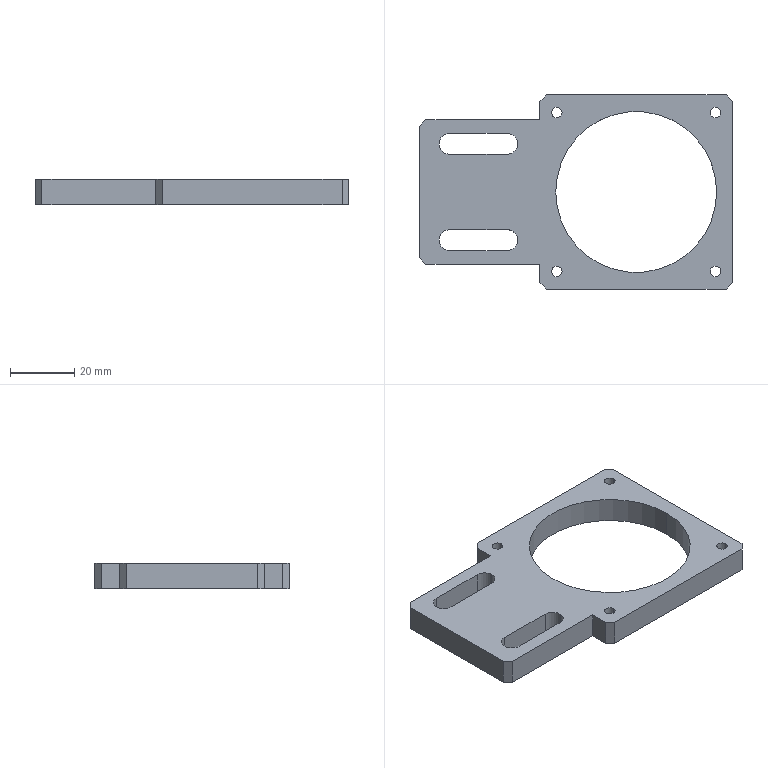Part | 1 solid | 44 faces | box 97.5 x 60.5 x 8 mm | volume 23818 mm3 | cylinder 20 | plane 20 | cone 4 | commonest cylinder face diameters 3.3 x12 6.5 x6 50.1 x2
STEP:
#1=CARTESIAN_POINT('',(-18.153,-15.,0.));
#2=VERTEX_POINT('',#1);
#3=CARTESIAN_POINT('',(-21.403,-18.25,0.));
#4=VERTEX_POINT('',#3);
#5=CARTESIAN_POINT('',(-21.403,-15.,0.));
#6=DIRECTION('',(0.,0.,-1.));
#7=DIRECTION('',(-1.,0.,0.));
#8=AXIS2_PLACEMENT_3D('',#5,#6,#7);
#9=CIRCLE('',#8,3.25);
#10=EDGE_CURVE('',#2,#4,#9,.T.);
#11=ORIENTED_EDGE('',*,*,#10,.F.);
#12=CARTESIAN_POINT('',(-18.153,-15.,-8.));
#13=VERTEX_POINT('',#12);
#14=CARTESIAN_POINT('',(-18.153,-15.,0.));
#15=DIRECTION('',(0.,0.,-1.));
#16=VECTOR('',#15,1000.);
#17=LINE('',#14,#16);
#18=EDGE_CURVE('',#2,#13,#17,.T.);
#19=ORIENTED_EDGE('',*,*,#18,.T.);
#20=CARTESIAN_POINT('',(-21.403,-18.25,-8.));
#21=VERTEX_POINT('',#20);
#22=CARTESIAN_POINT('',(-21.403,-15.,-8.));
#23=DIRECTION('',(0.,0.,-1.));
#24=DIRECTION('',(-1.,0.,0.));
#25=AXIS2_PLACEMENT_3D('',#22,#23,#24);
#26=CIRCLE('',#25,3.25);
#27=EDGE_CURVE('',#13,#21,#26,.T.);
#28=ORIENTED_EDGE('',*,*,#27,.T.);
#29=CARTESIAN_POINT('',(-21.403,-18.25,0.));
#30=DIRECTION('',(0.,0.,-1.));
#31=VECTOR('',#30,1000.);
#32=LINE('',#29,#31);
#33=EDGE_CURVE('',#4,#21,#32,.T.);
#34=ORIENTED_EDGE('',*,*,#33,.F.);
#35=EDGE_LOOP('',(#11,#19,#28,#34));
#36=FACE_BOUND('',#35,.T.);
#37=CARTESIAN_POINT('',(-21.403,-15.,0.));
#38=DIRECTION('',(0.,0.,-1.));
#39=DIRECTION('',(-1.,0.,0.));
#40=AXIS2_PLACEMENT_3D('',#37,#38,#39);
#41=CYLINDRICAL_SURFACE('',#40,3.25);
#42=ADVANCED_FACE('',(#36),#41,.F.);
#43=CARTESIAN_POINT('',(-18.153,15.,0.));
#44=VERTEX_POINT('',#43);
#45=CARTESIAN_POINT('',(-21.403,11.75,0.));
#46=VERTEX_POINT('',#45);
#47=CARTESIAN_POINT('',(-21.403,15.,0.));
#48=DIRECTION('',(0.,0.,-1.));
#49=DIRECTION('',(1.,0.,0.));
#50=AXIS2_PLACEMENT_3D('',#47,#48,#49);
#51=CIRCLE('',#50,3.25);
#52=EDGE_CURVE('',#44,#46,#51,.T.);
#53=ORIENTED_EDGE('',*,*,#52,.F.);
#54=CARTESIAN_POINT('',(-18.153,15.,-8.));
#55=VERTEX_POINT('',#54);
#56=CARTESIAN_POINT('',(-18.153,15.,0.));
#57=DIRECTION('',(0.,0.,-1.));
#58=VECTOR('',#57,1000.);
#59=LINE('',#56,#58);
#60=EDGE_CURVE('',#44,#55,#59,.T.);
#61=ORIENTED_EDGE('',*,*,#60,.T.);
#62=CARTESIAN_POINT('',(-21.403,11.75,-8.));
#63=VERTEX_POINT('',#62);
#64=CARTESIAN_POINT('',(-21.403,15.,-8.));
#65=DIRECTION('',(0.,0.,-1.));
#66=DIRECTION('',(1.,0.,0.));
#67=AXIS2_PLACEMENT_3D('',#64,#65,#66);
#68=CIRCLE('',#67,3.25);
#69=EDGE_CURVE('',#55,#63,#68,.T.);
#70=ORIENTED_EDGE('',*,*,#69,.T.);
#71=CARTESIAN_POINT('',(-21.403,11.75,0.));
#72=DIRECTION('',(0.,0.,-1.));
#73=VECTOR('',#72,1000.);
#74=LINE('',#71,#73);
#75=EDGE_CURVE('',#46,#63,#74,.T.);
#76=ORIENTED_EDGE('',*,*,#75,.F.);
#77=EDGE_LOOP('',(#53,#61,#70,#76));
#78=FACE_BOUND('',#77,.T.);
#79=CARTESIAN_POINT('',(-21.403,15.,0.));
#80=DIRECTION('',(0.,0.,-1.));
#81=DIRECTION('',(-1.,0.,0.));
#82=AXIS2_PLACEMENT_3D('',#79,#80,#81);
#83=CYLINDRICAL_SURFACE('',#82,3.25);
#84=ADVANCED_FACE('',(#78),#83,.F.);
#85=CARTESIAN_POINT('',(38.65,-21.65,-5.5));
#86=VERTEX_POINT('',#85);
#87=CARTESIAN_POINT('',(38.65,-18.35,-5.5));
#88=VERTEX_POINT('',#87);
#89=CARTESIAN_POINT('',(38.65,-20.,-5.5));
#90=DIRECTION('',(1.,0.,0.));
#91=DIRECTION('',(0.,1.,0.));
#92=AXIS2_PLACEMENT_3D('',#89,#90,#91);
#93=CIRCLE('',#92,1.65);
#94=EDGE_CURVE('',#86,#88,#93,.T.);
#95=ORIENTED_EDGE('',*,*,#94,.F.);
#96=CARTESIAN_POINT('',(48.75,-21.65,-5.5));
#97=VERTEX_POINT('',#96);
#98=CARTESIAN_POINT('',(48.75,-21.65,-5.5));
#99=DIRECTION('',(1.,0.,0.));
#100=VECTOR('',#99,1000.);
#101=LINE('',#98,#100);
#102=EDGE_CURVE('',#97,#86,#101,.F.);
#103=ORIENTED_EDGE('',*,*,#102,.F.);
#104=CARTESIAN_POINT('',(48.75,-18.35,-5.5));
#105=VERTEX_POINT('',#104);
#106=CARTESIAN_POINT('',(48.75,-20.,-5.5));
#107=DIRECTION('',(1.,0.,0.));
#108=DIRECTION('',(0.,1.,0.));
#109=AXIS2_PLACEMENT_3D('',#106,#107,#108);
#110=CIRCLE('',#109,1.65);
#111=EDGE_CURVE('',#97,#105,#110,.T.);
#112=ORIENTED_EDGE('',*,*,#111,.T.);
#113=CARTESIAN_POINT('',(48.75,-18.35,-5.5));
#114=DIRECTION('',(1.,0.,0.));
#115=VECTOR('',#114,1000.);
#116=LINE('',#113,#115);
#117=EDGE_CURVE('',#105,#88,#116,.F.);
#118=ORIENTED_EDGE('',*,*,#117,.T.);
#119=EDGE_LOOP('',(#95,#103,#112,#118));
#120=FACE_BOUND('',#119,.T.);
#121=CARTESIAN_POINT('',(48.75,-20.,-5.5));
#122=DIRECTION('',(1.,0.,0.));
#123=DIRECTION('',(0.,-1.,0.));
#124=AXIS2_PLACEMENT_3D('',#121,#122,#123);
#125=CYLINDRICAL_SURFACE('',#124,1.65);
#126=ADVANCED_FACE('',(#120),#125,.F.);
#127=CARTESIAN_POINT('',(37.659,-20.,-5.5));
#128=VERTEX_POINT('',#127);
#129=CARTESIAN_POINT('',(38.65,-18.35,-5.5));
#130=DIRECTION('',(0.515,0.8572,0.));
#131=VECTOR('',#130,1000.);
#132=LINE('',#129,#131);
#133=EDGE_CURVE('',#88,#128,#132,.F.);
#134=ORIENTED_EDGE('',*,*,#133,.T.);
#135=CARTESIAN_POINT('',(38.65,-21.65,-5.5));
#136=DIRECTION('',(0.515,-0.8572,0.));
#137=VECTOR('',#136,1000.);
#138=LINE('',#135,#137);
#139=EDGE_CURVE('',#86,#128,#138,.F.);
#140=ORIENTED_EDGE('',*,*,#139,.F.);
#141=ORIENTED_EDGE('',*,*,#94,.T.);
#142=EDGE_LOOP('',(#134,#140,#141));
#143=FACE_BOUND('',#142,.T.);
#144=CARTESIAN_POINT('',(38.65,-20.,-5.5));
#145=DIRECTION('',(1.,0.,0.));
#146=DIRECTION('',(0.,-1.,0.));
#147=AXIS2_PLACEMENT_3D('',#144,#145,#146);
#148=CONICAL_SURFACE('',#147,1.65,1.03);
#149=ADVANCED_FACE('',(#143),#148,.F.);
#150=CARTESIAN_POINT('',(38.65,18.35,-5.5));
#151=VERTEX_POINT('',#150);
#152=CARTESIAN_POINT('',(38.65,21.65,-5.5));
#153=VERTEX_POINT('',#152);
#154=CARTESIAN_POINT('',(38.65,20.,-5.5));
#155=DIRECTION('',(1.,0.,0.));
#156=DIRECTION('',(0.,1.,0.));
#157=AXIS2_PLACEMENT_3D('',#154,#155,#156);
#158=CIRCLE('',#157,1.65);
#159=EDGE_CURVE('',#151,#153,#158,.T.);
#160=ORIENTED_EDGE('',*,*,#159,.F.);
#161=CARTESIAN_POINT('',(48.75,18.35,-5.5));
#162=VERTEX_POINT('',#161);
#163=CARTESIAN_POINT('',(48.75,18.35,-5.5));
#164=DIRECTION('',(1.,0.,0.));
#165=VECTOR('',#164,1000.);
#166=LINE('',#163,#165);
#167=EDGE_CURVE('',#162,#151,#166,.F.);
#168=ORIENTED_EDGE('',*,*,#167,.F.);
#169=CARTESIAN_POINT('',(48.75,21.65,-5.5));
#170=VERTEX_POINT('',#169);
#171=CARTESIAN_POINT('',(48.75,20.,-5.5));
#172=DIRECTION('',(1.,0.,0.));
#173=DIRECTION('',(0.,1.,0.));
#174=AXIS2_PLACEMENT_3D('',#171,#172,#173);
#175=CIRCLE('',#174,1.65);
#176=EDGE_CURVE('',#162,#170,#175,.T.);
#177=ORIENTED_EDGE('',*,*,#176,.T.);
#178=CARTESIAN_POINT('',(48.75,21.65,-5.5));
#179=DIRECTION('',(1.,0.,0.));
#180=VECTOR('',#179,1000.);
#181=LINE('',#178,#180);
#182=EDGE_CURVE('',#170,#153,#181,.F.);
#183=ORIENTED_EDGE('',*,*,#182,.T.);
#184=EDGE_LOOP('',(#160,#168,#177,#183));
#185=FACE_BOUND('',#184,.T.);
#186=CARTESIAN_POINT('',(48.75,20.,-5.5));
#187=DIRECTION('',(1.,0.,0.));
#188=DIRECTION('',(0.,-1.,0.));
#189=AXIS2_PLACEMENT_3D('',#186,#187,#188);
#190=CYLINDRICAL_SURFACE('',#189,1.65);
#191=ADVANCED_FACE('',(#185),#190,.F.);
#192=CARTESIAN_POINT('',(37.659,20.,-5.5));
#193=VERTEX_POINT('',#192);
#194=CARTESIAN_POINT('',(38.65,21.65,-5.5));
#195=DIRECTION('',(0.515,0.8572,0.));
#196=VECTOR('',#195,1000.);
#197=LINE('',#194,#196);
#198=EDGE_CURVE('',#153,#193,#197,.F.);
#199=ORIENTED_EDGE('',*,*,#198,.T.);
#200=CARTESIAN_POINT('',(38.65,18.35,-5.5));
#201=DIRECTION('',(0.515,-0.8572,0.));
#202=VECTOR('',#201,1000.);
#203=LINE('',#200,#202);
#204=EDGE_CURVE('',#151,#193,#203,.F.);
#205=ORIENTED_EDGE('',*,*,#204,.F.);
#206=ORIENTED_EDGE('',*,*,#159,.T.);
#207=EDGE_LOOP('',(#199,#205,#206));
#208=FACE_BOUND('',#207,.T.);
#209=CARTESIAN_POINT('',(38.65,20.,-5.5));
#210=DIRECTION('',(1.,0.,0.));
#211=DIRECTION('',(0.,-1.,0.));
#212=AXIS2_PLACEMENT_3D('',#209,#210,#211);
#213=CONICAL_SURFACE('',#212,1.65,1.03);
#214=ADVANCED_FACE('',(#208),#213,.F.);
#215=CARTESIAN_POINT('',(-6.3,0.,0.));
#216=VERTEX_POINT('',#215);
#217=CARTESIAN_POINT('',(43.8,0.,0.));
#218=VERTEX_POINT('',#217);
#219=CARTESIAN_POINT('',(18.75,0.,0.));
#220=DIRECTION('',(0.,0.,-1.));
#221=DIRECTION('',(1.,0.,0.));
#222=AXIS2_PLACEMENT_3D('',#219,#220,#221);
#223=CIRCLE('',#222,25.05);
#224=EDGE_CURVE('',#216,#218,#223,.T.);
#225=ORIENTED_EDGE('',*,*,#224,.F.);
#226=CARTESIAN_POINT('',(-6.3,0.,-8.));
#227=VERTEX_POINT('',#226);
#228=CARTESIAN_POINT('',(-6.3,0.,0.));
#229=DIRECTION('',(0.,0.,-1.));
#230=VECTOR('',#229,1000.);
#231=LINE('',#228,#230);
#232=EDGE_CURVE('',#227,#216,#231,.F.);
#233=ORIENTED_EDGE('',*,*,#232,.F.);
#234=CARTESIAN_POINT('',(43.8,0.,-8.));
#235=VERTEX_POINT('',#234);
#236=CARTESIAN_POINT('',(18.75,0.,-8.));
#237=DIRECTION('',(0.,0.,-1.));
#238=DIRECTION('',(1.,0.,0.));
#239=AXIS2_PLACEMENT_3D('',#236,#237,#238);
#240=CIRCLE('',#239,25.05);
#241=EDGE_CURVE('',#227,#235,#240,.T.);
#242=ORIENTED_EDGE('',*,*,#241,.T.);
#243=CARTESIAN_POINT('',(43.8,0.,0.));
#244=DIRECTION('',(0.,0.,-1.));
#245=VECTOR('',#244,1000.);
#246=LINE('',#243,#245);
#247=EDGE_CURVE('',#235,#218,#246,.F.);
#248=ORIENTED_EDGE('',*,*,#247,.T.);
#249=EDGE_LOOP('',(#225,#233,#242,#248));
#250=FACE_BOUND('',#249,.T.);
#251=CARTESIAN_POINT('',(18.75,0.,0.));
#252=DIRECTION('',(0.,0.,-1.));
#253=DIRECTION('',(-1.,0.,0.));
#254=AXIS2_PLACEMENT_3D('',#251,#252,#253);
#255=CYLINDRICAL_SURFACE('',#254,25.05);
#256=ADVANCED_FACE('',(#250),#255,.F.);
#257=CARTESIAN_POINT('',(45.149,24.749,0.));
#258=VERTEX_POINT('',#257);
#259=CARTESIAN_POINT('',(41.849,24.749,0.));
#260=VERTEX_POINT('',#259);
#261=CARTESIAN_POINT('',(43.499,24.749,0.));
#262=DIRECTION('',(0.,0.,1.));
#263=DIRECTION('',(-1.,0.,0.));
#264=AXIS2_PLACEMENT_3D('',#261,#262,#263);
#265=CIRCLE('',#264,1.65);
#266=EDGE_CURVE('',#258,#260,#265,.T.);
#267=ORIENTED_EDGE('',*,*,#266,.T.);
#268=CARTESIAN_POINT('',(41.849,24.749,-8.));
#269=VERTEX_POINT('',#268);
#270=CARTESIAN_POINT('',(41.849,24.749,-8.));
#271=DIRECTION('',(0.,0.,-1.));
#272=VECTOR('',#271,1000.);
#273=LINE('',#270,#272);
#274=EDGE_CURVE('',#269,#260,#273,.F.);
#275=ORIENTED_EDGE('',*,*,#274,.F.);
#276=CARTESIAN_POINT('',(45.149,24.749,-8.));
#277=VERTEX_POINT('',#276);
#278=CARTESIAN_POINT('',(43.499,24.749,-8.));
#279=DIRECTION('',(0.,0.,-1.));
#280=DIRECTION('',(1.,0.,0.));
#281=AXIS2_PLACEMENT_3D('',#278,#279,#280);
#282=CIRCLE('',#281,1.65);
#283=EDGE_CURVE('',#269,#277,#282,.T.);
#284=ORIENTED_EDGE('',*,*,#283,.T.);
#285=CARTESIAN_POINT('',(45.149,24.749,-8.));
#286=DIRECTION('',(0.,0.,-1.));
#287=VECTOR('',#286,1000.);
#288=LINE('',#285,#287);
#289=EDGE_CURVE('',#277,#258,#288,.F.);
#290=ORIENTED_EDGE('',*,*,#289,.T.);
#291=EDGE_LOOP('',(#267,#275,#284,#290));
#292=FACE_BOUND('',#291,.T.);
#293=CARTESIAN_POINT('',(43.499,24.749,-8.));
#294=DIRECTION('',(0.,0.,-1.));
#295=DIRECTION('',(-1.,0.,0.));
#296=AXIS2_PLACEMENT_3D('',#293,#294,#295);
#297=CYLINDRICAL_SURFACE('',#296,1.65);
#298=ADVANCED_FACE('',(#292),#297,.F.);
#299=CARTESIAN_POINT('',(45.149,-24.749,0.));
#300=VERTEX_POINT('',#299);
#301=CARTESIAN_POINT('',(41.849,-24.749,0.));
#302=VERTEX_POINT('',#301);
#303=CARTESIAN_POINT('',(43.499,-24.749,0.));
#304=DIRECTION('',(0.,0.,1.));
#305=DIRECTION('',(-1.,0.,0.));
#306=AXIS2_PLACEMENT_3D('',#303,#304,#305);
#307=CIRCLE('',#306,1.65);
#308=EDGE_CURVE('',#300,#302,#307,.T.);
#309=ORIENTED_EDGE('',*,*,#308,.T.);
#310=CARTESIAN_POINT('',(41.849,-24.749,-8.));
#311=VERTEX_POINT('',#310);
#312=CARTESIAN_POINT('',(41.849,-24.749,-8.));
#313=DIRECTION('',(0.,0.,-1.));
#314=VECTOR('',#313,1000.);
#315=LINE('',#312,#314);
#316=EDGE_CURVE('',#311,#302,#315,.F.);
#317=ORIENTED_EDGE('',*,*,#316,.F.);
#318=CARTESIAN_POINT('',(45.149,-24.749,-8.));
#319=VERTEX_POINT('',#318);
#320=CARTESIAN_POINT('',(43.499,-24.749,-8.));
#321=DIRECTION('',(0.,0.,-1.));
#322=DIRECTION('',(1.,0.,0.));
#323=AXIS2_PLACEMENT_3D('',#320,#321,#322);
#324=CIRCLE('',#323,1.65);
#325=EDGE_CURVE('',#311,#319,#324,.T.);
#326=ORIENTED_EDGE('',*,*,#325,.T.);
#327=CARTESIAN_POINT('',(45.149,-24.749,-8.));
#328=DIRECTION('',(0.,0.,-1.));
#329=VECTOR('',#328,1000.);
#330=LINE('',#327,#329);
#331=EDGE_CURVE('',#319,#300,#330,.F.);
#332=ORIENTED_EDGE('',*,*,#331,.T.);
#333=EDGE_LOOP('',(#309,#317,#326,#332));
#334=FACE_BOUND('',#333,.T.);
#335=CARTESIAN_POINT('',(43.499,-24.749,-8.));
#336=DIRECTION('',(0.,0.,-1.));
#337=DIRECTION('',(-1.,0.,0.));
#338=AXIS2_PLACEMENT_3D('',#335,#336,#337);
#339=CYLINDRICAL_SURFACE('',#338,1.65);
#340=ADVANCED_FACE('',(#334),#339,.F.);
#341=CARTESIAN_POINT('',(-4.349,-24.749,0.));
#342=VERTEX_POINT('',#341);
#343=CARTESIAN_POINT('',(-7.649,-24.749,0.));
#344=VERTEX_POINT('',#343);
#345=CARTESIAN_POINT('',(-5.999,-24.749,0.));
#346=DIRECTION('',(0.,0.,1.));
#347=DIRECTION('',(-1.,0.,0.));
#348=AXIS2_PLACEMENT_3D('',#345,#346,#347);
#349=CIRCLE('',#348,1.65);
#350=EDGE_CURVE('',#342,#344,#349,.T.);
#351=ORIENTED_EDGE('',*,*,#350,.T.);
#352=CARTESIAN_POINT('',(-7.649,-24.749,-8.));
#353=VERTEX_POINT('',#352);
#354=CARTESIAN_POINT('',(-7.649,-24.749,-8.));
#355=DIRECTION('',(0.,0.,-1.));
#356=VECTOR('',#355,1000.);
#357=LINE('',#354,#356);
#358=EDGE_CURVE('',#353,#344,#357,.F.);
#359=ORIENTED_EDGE('',*,*,#358,.F.);
#360=CARTESIAN_POINT('',(-4.349,-24.749,-8.));
#361=VERTEX_POINT('',#360);
#362=CARTESIAN_POINT('',(-5.999,-24.749,-8.));
#363=DIRECTION('',(0.,0.,-1.));
#364=DIRECTION('',(1.,0.,0.));
#365=AXIS2_PLACEMENT_3D('',#362,#363,#364);
#366=CIRCLE('',#365,1.65);
#367=EDGE_CURVE('',#353,#361,#366,.T.);
#368=ORIENTED_EDGE('',*,*,#367,.T.);
#369=CARTESIAN_POINT('',(-4.349,-24.749,-8.));
#370=DIRECTION('',(0.,0.,-1.));
#371=VECTOR('',#370,1000.);
#372=LINE('',#369,#371);
#373=EDGE_CURVE('',#361,#342,#372,.F.);
#374=ORIENTED_EDGE('',*,*,#373,.T.);
#375=EDGE_LOOP('',(#351,#359,#368,#374));
#376=FACE_BOUND('',#375,.T.);
#377=CARTESIAN_POINT('',(-5.999,-24.749,-8.));
#378=DIRECTION('',(0.,0.,-1.));
#379=DIRECTION('',(-1.,0.,0.));
#380=AXIS2_PLACEMENT_3D('',#377,#378,#379);
#381=CYLINDRICAL_SURFACE('',#380,1.65);
#382=ADVANCED_FACE('',(#376),#381,.F.);
#383=CARTESIAN_POINT('',(-4.349,24.749,0.));
#384=VERTEX_POINT('',#383);
#385=CARTESIAN_POINT('',(-7.649,24.749,0.));
#386=VERTEX_POINT('',#385);
#387=CARTESIAN_POINT('',(-5.999,24.749,0.));
#388=DIRECTION('',(0.,0.,1.));
#389=DIRECTION('',(-1.,0.,0.));
#390=AXIS2_PLACEMENT_3D('',#387,#388,#389);
#391=CIRCLE('',#390,1.65);
#392=EDGE_CURVE('',#384,#386,#391,.T.);
#393=ORIENTED_EDGE('',*,*,#392,.T.);
#394=CARTESIAN_POINT('',(-7.649,24.749,-8.));
#395=VERTEX_POINT('',#394);
#396=CARTESIAN_POINT('',(-7.649,24.749,-8.));
#397=DIRECTION('',(0.,0.,-1.));
#398=VECTOR('',#397,1000.);
#399=LINE('',#396,#398);
#400=EDGE_CURVE('',#395,#386,#399,.F.);
#401=ORIENTED_EDGE('',*,*,#400,.F.);
#402=CARTESIAN_POINT('',(-4.349,24.749,-8.));
#403=VERTEX_POINT('',#402);
#404=CARTESIAN_POINT('',(-5.999,24.749,-8.));
#405=DIRECTION('',(0.,0.,-1.));
#406=DIRECTION('',(1.,0.,0.));
#407=AXIS2_PLACEMENT_3D('',#404,#405,#406);
#408=CIRCLE('',#407,1.65);
#409=EDGE_CURVE('',#395,#403,#408,.T.);
#410=ORIENTED_EDGE('',*,*,#409,.T.);
#411=CARTESIAN_POINT('',(-4.349,24.749,-8.));
#412=DIRECTION('',(0.,0.,-1.));
#413=VECTOR('',#412,1000.);
#414=LINE('',#411,#413);
#415=EDGE_CURVE('',#403,#384,#414,.F.);
#416=ORIENTED_EDGE('',*,*,#415,.T.);
#417=EDGE_LOOP('',(#393,#401,#410,#416));
#418=FACE_BOUND('',#417,.T.);
#419=CARTESIAN_POINT('',(-5.999,24.749,-8.));
#420=DIRECTION('',(0.,0.,-1.));
#421=DIRECTION('',(-1.,0.,0.));
#422=AXIS2_PLACEMENT_3D('',#419,#420,#421);
#423=CYLINDRICAL_SURFACE('',#422,1.65);
#424=ADVANCED_FACE('',(#418),#423,.F.);
#425=CARTESIAN_POINT('',(-39.403,-11.75,-8.));
#426=VERTEX_POINT('',#425);
#427=CARTESIAN_POINT('',(-21.403,-11.75,-8.));
#428=VERTEX_POINT('',#427);
#429=CARTESIAN_POINT('',(-39.403,-11.75,-8.));
#430=DIRECTION('',(1.,0.,0.));
#431=VECTOR('',#430,1000.);
#432=LINE('',#429,#431);
#433=EDGE_CURVE('',#426,#428,#432,.T.);
#434=ORIENTED_EDGE('',*,*,#433,.F.);
#435=CARTESIAN_POINT('',(-39.403,-18.25,-8.));
#436=VERTEX_POINT('',#435);
#437=CARTESIAN_POINT('',(-39.403,-15.,-8.));
#438=DIRECTION('',(0.,0.,-1.));
#439=DIRECTION('',(-1.,0.,0.));
#440=AXIS2_PLACEMENT_3D('',#437,#438,#439);
#441=CIRCLE('',#440,3.25);
#442=EDGE_CURVE('',#436,#426,#441,.T.);
#443=ORIENTED_EDGE('',*,*,#442,.F.);
#444=CARTESIAN_POINT('',(-39.403,-18.25,-8.));
#445=DIRECTION('',(-1.,0.,0.));
#446=VECTOR('',#445,1000.);
#447=LINE('',#444,#446);
#448=EDGE_CURVE('',#21,#436,#447,.T.);
#449=ORIENTED_EDGE('',*,*,#448,.F.);
#450=ORIENTED_EDGE('',*,*,#27,.F.);
#451=CARTESIAN_POINT('',(-21.403,-15.,-8.));
#452=DIRECTION('',(0.,0.,-1.));
#453=DIRECTION('',(-1.,0.,0.));
#454=AXIS2_PLACEMENT_3D('',#451,#452,#453);
#455=CIRCLE('',#454,3.25);
#456=EDGE_CURVE('',#428,#13,#455,.T.);
#457=ORIENTED_EDGE('',*,*,#456,.F.);
#458=EDGE_LOOP('',(#434,#443,#449,#450,#457));
#459=FACE_BOUND('',#458,.T.);
#460=CARTESIAN_POINT('',(-39.403,18.25,-8.));
#461=VERTEX_POINT('',#460);
#462=CARTESIAN_POINT('',(-21.403,18.25,-8.));
#463=VERTEX_POINT('',#462);
#464=CARTESIAN_POINT('',(-39.403,18.25,-8.));
#465=DIRECTION('',(1.,0.,0.));
#466=VECTOR('',#465,1000.);
#467=LINE('',#464,#466);
#468=EDGE_CURVE('',#461,#463,#467,.T.);
#469=ORIENTED_EDGE('',*,*,#468,.F.);
#470=CARTESIAN_POINT('',(-39.403,11.75,-8.));
#471=VERTEX_POINT('',#470);
#472=CARTESIAN_POINT('',(-39.403,15.,-8.));
#473=DIRECTION('',(0.,0.,-1.));
#474=DIRECTION('',(1.,0.,0.));
#475=AXIS2_PLACEMENT_3D('',#472,#473,#474);
#476=CIRCLE('',#475,3.25);
#477=EDGE_CURVE('',#471,#461,#476,.T.);
#478=ORIENTED_EDGE('',*,*,#477,.F.);
#479=CARTESIAN_POINT('',(-39.403,11.75,-8.));
#480=DIRECTION('',(-1.,0.,0.));
#481=VECTOR('',#480,1000.);
#482=LINE('',#479,#481);
#483=EDGE_CURVE('',#63,#471,#482,.T.);
#484=ORIENTED_EDGE('',*,*,#483,.F.);
#485=ORIENTED_EDGE('',*,*,#69,.F.);
#486=CARTESIAN_POINT('',(-21.403,15.,-8.));
#487=DIRECTION('',(0.,0.,-1.));
#488=DIRECTION('',(1.,0.,0.));
#489=AXIS2_PLACEMENT_3D('',#486,#487,#488);
#490=CIRCLE('',#489,3.25);
#491=EDGE_CURVE('',#463,#55,#490,.T.);
#492=ORIENTED_EDGE('',*,*,#491,.F.);
#493=EDGE_LOOP('',(#469,#478,#484,#485,#492));
#494=FACE_BOUND('',#493,.T.);
#495=CARTESIAN_POINT('',(18.75,0.,-8.));
#496=DIRECTION('',(0.,0.,-1.));
#497=DIRECTION('',(1.,0.,0.));
#498=AXIS2_PLACEMENT_3D('',#495,#496,#497);
#499=CIRCLE('',#498,25.05);
#500=EDGE_CURVE('',#235,#227,#499,.T.);
#501=ORIENTED_EDGE('',*,*,#500,.F.);
#502=ORIENTED_EDGE('',*,*,#241,.F.);
#503=EDGE_LOOP('',(#501,#502));
#504=FACE_BOUND('',#503,.T.);
#505=CARTESIAN_POINT('',(43.499,24.749,-8.));
#506=DIRECTION('',(0.,0.,-1.));
#507=DIRECTION('',(1.,0.,0.));
#508=AXIS2_PLACEMENT_3D('',#505,#506,#507);
#509=CIRCLE('',#508,1.65);
#510=EDGE_CURVE('',#277,#269,#509,.T.);
#511=ORIENTED_EDGE('',*,*,#510,.F.);
#512=ORIENTED_EDGE('',*,*,#283,.F.);
#513=EDGE_LOOP('',(#511,#512));
#514=FACE_BOUND('',#513,.T.);
#515=CARTESIAN_POINT('',(43.499,-24.749,-8.));
#516=DIRECTION('',(0.,0.,-1.));
#517=DIRECTION('',(1.,0.,0.));
#518=AXIS2_PLACEMENT_3D('',#515,#516,#517);
#519=CIRCLE('',#518,1.65);
#520=EDGE_CURVE('',#319,#311,#519,.T.);
#521=ORIENTED_EDGE('',*,*,#520,.F.);
#522=ORIENTED_EDGE('',*,*,#325,.F.);
#523=EDGE_LOOP('',(#521,#522));
#524=FACE_BOUND('',#523,.T.);
#525=CARTESIAN_POINT('',(-5.999,24.749,-8.));
#526=DIRECTION('',(0.,0.,-1.));
#527=DIRECTION('',(1.,0.,0.));
#528=AXIS2_PLACEMENT_3D('',#525,#526,#527);
#529=CIRCLE('',#528,1.65);
#530=EDGE_CURVE('',#403,#395,#529,.T.);
#531=ORIENTED_EDGE('',*,*,#530,.F.);
#532=ORIENTED_EDGE('',*,*,#409,.F.);
#533=EDGE_LOOP('',(#531,#532));
#534=FACE_BOUND('',#533,.T.);
#535=CARTESIAN_POINT('',(-48.75,20.5,-8.));
#536=VERTEX_POINT('',#535);
#537=CARTESIAN_POINT('',(-48.75,-20.5,-8.));
#538=VERTEX_POINT('',#537);
#539=CARTESIAN_POINT('',(-48.75,30.25,-8.));
#540=DIRECTION('',(0.,-1.,0.));
#541=VECTOR('',#540,1000.);
#542=LINE('',#539,#541);
#543=EDGE_CURVE('',#536,#538,#542,.T.);
#544=ORIENTED_EDGE('',*,*,#543,.F.);
#545=CARTESIAN_POINT('',(-46.75,22.5,-8.));
#546=VERTEX_POINT('',#545);
#547=CARTESIAN_POINT('',(-48.75,20.5,-8.));
#548=DIRECTION('',(0.7071,0.7071,0.));
#549=VECTOR('',#548,1000.);
#550=LINE('',#547,#549);
#551=EDGE_CURVE('',#536,#546,#550,.T.);
#552=ORIENTED_EDGE('',*,*,#551,.T.);
#553=CARTESIAN_POINT('',(-11.25,22.5,-8.));
#554=VERTEX_POINT('',#553);
#555=CARTESIAN_POINT('',(-48.75,22.5,-8.));
#556=DIRECTION('',(-1.,0.,0.));
#557=VECTOR('',#556,1000.);
#558=LINE('',#555,#557);
#559=EDGE_CURVE('',#554,#546,#558,.T.);
#560=ORIENTED_EDGE('',*,*,#559,.F.);
#561=CARTESIAN_POINT('',(-11.25,28.25,-8.));
#562=VERTEX_POINT('',#561);
#563=CARTESIAN_POINT('',(-11.25,30.25,-8.));
#564=DIRECTION('',(0.,-1.,0.));
#565=VECTOR('',#564,1000.);
#566=LINE('',#563,#565);
#567=EDGE_CURVE('',#562,#554,#566,.T.);
#568=ORIENTED_EDGE('',*,*,#567,.F.);
#569=CARTESIAN_POINT('',(-9.25,30.25,-8.));
#570=VERTEX_POINT('',#569);
#571=CARTESIAN_POINT('',(-11.25,28.25,-8.));
#572=DIRECTION('',(0.7071,0.7071,0.));
#573=VECTOR('',#572,1000.);
#574=LINE('',#571,#573);
#575=EDGE_CURVE('',#562,#570,#574,.T.);
#576=ORIENTED_EDGE('',*,*,#575,.T.);
#577=CARTESIAN_POINT('',(46.75,30.25,-8.));
#578=VERTEX_POINT('',#577);
#579=CARTESIAN_POINT('',(48.75,30.25,-8.));
#580=DIRECTION('',(-1.,0.,0.));
#581=VECTOR('',#580,1000.);
#582=LINE('',#579,#581);
#583=EDGE_CURVE('',#578,#570,#582,.T.);
#584=ORIENTED_EDGE('',*,*,#583,.F.);
#585=CARTESIAN_POINT('',(48.75,28.25,-8.));
#586=VERTEX_POINT('',#585);
#587=CARTESIAN_POINT('',(46.75,30.25,-8.));
#588=DIRECTION('',(0.7071,-0.7071,0.));
#589=VECTOR('',#588,1000.);
#590=LINE('',#587,#589);
#591=EDGE_CURVE('',#578,#586,#590,.T.);
#592=ORIENTED_EDGE('',*,*,#591,.T.);
#593=CARTESIAN_POINT('',(48.75,-28.25,-8.));
#594=VERTEX_POINT('',#593);
#595=CARTESIAN_POINT('',(48.75,30.25,-8.));
#596=DIRECTION('',(0.,1.,0.));
#597=VECTOR('',#596,1000.);
#598=LINE('',#595,#597);
#599=EDGE_CURVE('',#594,#586,#598,.T.);
#600=ORIENTED_EDGE('',*,*,#599,.F.);
#601=CARTESIAN_POINT('',(46.75,-30.25,-8.));
#602=VERTEX_POINT('',#601);
#603=CARTESIAN_POINT('',(48.75,-28.25,-8.));
#604=DIRECTION('',(-0.7071,-0.7071,0.));
#605=VECTOR('',#604,1000.);
#606=LINE('',#603,#605);
#607=EDGE_CURVE('',#594,#602,#606,.T.);
#608=ORIENTED_EDGE('',*,*,#607,.T.);
#609=CARTESIAN_POINT('',(-9.25,-30.25,-8.));
#610=VERTEX_POINT('',#609);
#611=CARTESIAN_POINT('',(48.75,-30.25,-8.));
#612=DIRECTION('',(1.,0.,0.));
#613=VECTOR('',#612,1000.);
#614=LINE('',#611,#613);
#615=EDGE_CURVE('',#610,#602,#614,.T.);
#616=ORIENTED_EDGE('',*,*,#615,.F.);
#617=CARTESIAN_POINT('',(-11.25,-28.25,-8.));
#618=VERTEX_POINT('',#617);
#619=CARTESIAN_POINT('',(-9.25,-30.25,-8.));
#620=DIRECTION('',(-0.7071,0.7071,0.));
#621=VECTOR('',#620,1000.);
#622=LINE('',#619,#621);
#623=EDGE_CURVE('',#610,#618,#622,.T.);
#624=ORIENTED_EDGE('',*,*,#623,.T.);
#625=CARTESIAN_POINT('',(-11.25,-22.5,-8.));
#626=VERTEX_POINT('',#625);
#627=CARTESIAN_POINT('',(-11.25,-30.25,-8.));
#628=DIRECTION('',(0.,-1.,0.));
#629=VECTOR('',#628,1000.);
#630=LINE('',#627,#629);
#631=EDGE_CURVE('',#626,#618,#630,.T.);
#632=ORIENTED_EDGE('',*,*,#631,.F.);
#633=CARTESIAN_POINT('',(-46.75,-22.5,-8.));
#634=VERTEX_POINT('',#633);
#635=CARTESIAN_POINT('',(-48.75,-22.5,-8.));
#636=DIRECTION('',(1.,0.,0.));
#637=VECTOR('',#636,1000.);
#638=LINE('',#635,#637);
#639=EDGE_CURVE('',#634,#626,#638,.T.);
#640=ORIENTED_EDGE('',*,*,#639,.F.);
#641=CARTESIAN_POINT('',(-46.75,-22.5,-8.));
#642=DIRECTION('',(-0.7071,0.7071,0.));
#643=VECTOR('',#642,1000.);
#644=LINE('',#641,#643);
#645=EDGE_CURVE('',#634,#538,#644,.T.);
#646=ORIENTED_EDGE('',*,*,#645,.T.);
#647=EDGE_LOOP('',(#544,#552,#560,#568,#576,#584,#592,#600,#608,#616,#624,#632,#640,#646));
#648=FACE_BOUND('',#647,.T.);
#649=CARTESIAN_POINT('',(-5.999,-24.749,-8.));
#650=DIRECTION('',(0.,0.,-1.));
#651=DIRECTION('',(1.,0.,0.));
#652=AXIS2_PLACEMENT_3D('',#649,#650,#651);
#653=CIRCLE('',#652,1.65);
#654=EDGE_CURVE('',#361,#353,#653,.T.);
#655=ORIENTED_EDGE('',*,*,#654,.F.);
#656=ORIENTED_EDGE('',*,*,#367,.F.);
#657=EDGE_LOOP('',(#655,#656));
#658=FACE_BOUND('',#657,.T.);
#659=CARTESIAN_POINT('',(-48.75,30.25,-8.));
#660=DIRECTION('',(0.,0.,1.));
#661=DIRECTION('',(1.,0.,0.));
#662=AXIS2_PLACEMENT_3D('',#659,#660,#661);
#663=PLANE('',#662);
#664=ADVANCED_FACE('',(#459,#494,#504,#514,#524,#534,#648,#658),#663,.F.);
#665=ORIENTED_EDGE('',*,*,#583,.T.);
#666=CARTESIAN_POINT('',(-9.25,30.25,0.));
#667=VERTEX_POINT('',#666);
#668=CARTESIAN_POINT('',(-9.25,30.25,0.));
#669=DIRECTION('',(0.,0.,1.));
#670=VECTOR('',#669,1000.);
#671=LINE('',#668,#670);
#672=EDGE_CURVE('',#570,#667,#671,.T.);
#673=ORIENTED_EDGE('',*,*,#672,.T.);
#674=CARTESIAN_POINT('',(46.75,30.25,0.));
#675=VERTEX_POINT('',#674);
#676=CARTESIAN_POINT('',(48.75,30.25,0.));
#677=DIRECTION('',(-1.,0.,0.));
#678=VECTOR('',#677,1000.);
#679=LINE('',#676,#678);
#680=EDGE_CURVE('',#675,#667,#679,.T.);
#681=ORIENTED_EDGE('',*,*,#680,.F.);
#682=CARTESIAN_POINT('',(46.75,30.25,0.));
#683=DIRECTION('',(0.,0.,-1.));
#684=VECTOR('',#683,1000.);
#685=LINE('',#682,#684);
#686=EDGE_CURVE('',#675,#578,#685,.T.);
#687=ORIENTED_EDGE('',*,*,#686,.T.);
#688=EDGE_LOOP('',(#665,#673,#681,#687));
#689=FACE_BOUND('',#688,.T.);
#690=CARTESIAN_POINT('',(48.75,30.25,0.));
#691=DIRECTION('',(0.,-1.,0.));
#692=DIRECTION('',(-1.,0.,0.));
#693=AXIS2_PLACEMENT_3D('',#690,#691,#692);
#694=PLANE('',#693);
#695=ADVANCED_FACE('',(#689),#694,.F.);
#696=CARTESIAN_POINT('',(-48.75,20.5,0.));
#697=VERTEX_POINT('',#696);
#698=CARTESIAN_POINT('',(-48.75,-20.5,0.));
#699=VERTEX_POINT('',#698);
#700=CARTESIAN_POINT('',(-48.75,30.25,0.));
#701=DIRECTION('',(0.,-1.,0.));
#702=VECTOR('',#701,1000.);
#703=LINE('',#700,#702);
#704=EDGE_CURVE('',#697,#699,#703,.T.);
#705=ORIENTED_EDGE('',*,*,#704,.F.);
#706=CARTESIAN_POINT('',(-48.75,20.5,0.));
#707=DIRECTION('',(0.,0.,-1.));
#708=VECTOR('',#707,1000.);
#709=LINE('',#706,#708);
#710=EDGE_CURVE('',#697,#536,#709,.T.);
#711=ORIENTED_EDGE('',*,*,#710,.T.);
#712=ORIENTED_EDGE('',*,*,#543,.T.);
#713=CARTESIAN_POINT('',(-48.75,-20.5,0.));
#714=DIRECTION('',(0.,0.,1.));
#715=VECTOR('',#714,1000.);
#716=LINE('',#713,#715);
#717=EDGE_CURVE('',#538,#699,#716,.T.);
#718=ORIENTED_EDGE('',*,*,#717,.T.);
#719=EDGE_LOOP('',(#705,#711,#712,#718));
#720=FACE_BOUND('',#719,.T.);
#721=CARTESIAN_POINT('',(-48.75,30.25,0.));
#722=DIRECTION('',(1.,0.,0.));
#723=DIRECTION('',(0.,-1.,0.));
#724=AXIS2_PLACEMENT_3D('',#721,#722,#723);
#725=PLANE('',#724);
#726=ADVANCED_FACE('',(#720),#725,.F.);
#727=CARTESIAN_POINT('',(-9.25,-30.25,0.));
#728=VERTEX_POINT('',#727);
#729=CARTESIAN_POINT('',(46.75,-30.25,0.));
#730=VERTEX_POINT('',#729);
#731=CARTESIAN_POINT('',(48.75,-30.25,0.));
#732=DIRECTION('',(1.,0.,0.));
#733=VECTOR('',#732,1000.);
#734=LINE('',#731,#733);
#735=EDGE_CURVE('',#728,#730,#734,.T.);
#736=ORIENTED_EDGE('',*,*,#735,.F.);
#737=CARTESIAN_POINT('',(-9.25,-30.25,0.));
#738=DIRECTION('',(0.,0.,-1.));
#739=VECTOR('',#738,1000.);
#740=LINE('',#737,#739);
#741=EDGE_CURVE('',#728,#610,#740,.T.);
#742=ORIENTED_EDGE('',*,*,#741,.T.);
#743=ORIENTED_EDGE('',*,*,#615,.T.);
#744=CARTESIAN_POINT('',(46.75,-30.25,0.));
#745=DIRECTION('',(0.,0.,1.));
#746=VECTOR('',#745,1000.);
#747=LINE('',#744,#746);
#748=EDGE_CURVE('',#602,#730,#747,.T.);
#749=ORIENTED_EDGE('',*,*,#748,.T.);
#750=EDGE_LOOP('',(#736,#742,#743,#749));
#751=FACE_BOUND('',#750,.T.);
#752=CARTESIAN_POINT('',(48.75,-30.25,0.));
#753=DIRECTION('',(0.,1.,0.));
#754=DIRECTION('',(1.,0.,0.));
#755=AXIS2_PLACEMENT_3D('',#752,#753,#754);
#756=PLANE('',#755);
#757=ADVANCED_FACE('',(#751),#756,.F.);
#758=CARTESIAN_POINT('',(48.75,-20.,-5.5));
#759=DIRECTION('',(1.,0.,0.));
#760=DIRECTION('',(0.,1.,0.));
#761=AXIS2_PLACEMENT_3D('',#758,#759,#760);
#762=CIRCLE('',#761,1.65);
#763=EDGE_CURVE('',#105,#97,#762,.T.);
#764=ORIENTED_EDGE('',*,*,#763,.F.);
#765=ORIENTED_EDGE('',*,*,#111,.F.);
#766=EDGE_LOOP('',(#764,#765));
#767=FACE_BOUND('',#766,.T.);
#768=CARTESIAN_POINT('',(48.75,20.,-5.5));
#769=DIRECTION('',(1.,0.,0.));
#770=DIRECTION('',(0.,1.,0.));
#771=AXIS2_PLACEMENT_3D('',#768,#769,#770);
#772=CIRCLE('',#771,1.65);
#773=EDGE_CURVE('',#170,#162,#772,.T.);
#774=ORIENTED_EDGE('',*,*,#773,.F.);
#775=ORIENTED_EDGE('',*,*,#176,.F.);
#776=EDGE_LOOP('',(#774,#775));
#777=FACE_BOUND('',#776,.T.);
#778=CARTESIAN_POINT('',(48.75,-28.25,0.));
#779=VERTEX_POINT('',#778);
#780=CARTESIAN_POINT('',(48.75,28.25,0.));
#781=VERTEX_POINT('',#780);
#782=CARTESIAN_POINT('',(48.75,30.25,0.));
#783=DIRECTION('',(0.,1.,0.));
#784=VECTOR('',#783,1000.);
#785=LINE('',#782,#784);
#786=EDGE_CURVE('',#779,#781,#785,.T.);
#787=ORIENTED_EDGE('',*,*,#786,.F.);
#788=CARTESIAN_POINT('',(48.75,-28.25,0.));
#789=DIRECTION('',(0.,0.,-1.));
#790=VECTOR('',#789,1000.);
#791=LINE('',#788,#790);
#792=EDGE_CURVE('',#779,#594,#791,.T.);
#793=ORIENTED_EDGE('',*,*,#792,.T.);
#794=ORIENTED_EDGE('',*,*,#599,.T.);
#795=CARTESIAN_POINT('',(48.75,28.25,0.));
#796=DIRECTION('',(0.,0.,1.));
#797=VECTOR('',#796,1000.);
#798=LINE('',#795,#797);
#799=EDGE_CURVE('',#586,#781,#798,.T.);
#800=ORIENTED_EDGE('',*,*,#799,.T.);
#801=EDGE_LOOP('',(#787,#793,#794,#800));
#802=FACE_BOUND('',#801,.T.);
#803=CARTESIAN_POINT('',(48.75,30.25,0.));
#804=DIRECTION('',(-1.,0.,0.));
#805=DIRECTION('',(0.,1.,0.));
#806=AXIS2_PLACEMENT_3D('',#803,#804,#805);
#807=PLANE('',#806);
#808=ADVANCED_FACE('',(#767,#777,#802),#807,.F.);
#809=CARTESIAN_POINT('',(-39.403,-18.25,0.));
#810=VERTEX_POINT('',#809);
#811=CARTESIAN_POINT('',(-39.403,-11.75,0.));
#812=VERTEX_POINT('',#811);
#813=CARTESIAN_POINT('',(-39.403,-15.,0.));
#814=DIRECTION('',(0.,0.,-1.));
#815=DIRECTION('',(-1.,0.,0.));
#816=AXIS2_PLACEMENT_3D('',#813,#814,#815);
#817=CIRCLE('',#816,3.25);
#818=EDGE_CURVE('',#810,#812,#817,.T.);
#819=ORIENTED_EDGE('',*,*,#818,.T.);
#820=CARTESIAN_POINT('',(-21.403,-11.75,0.));
#821=VERTEX_POINT('',#820);
#822=CARTESIAN_POINT('',(-39.403,-11.75,0.));
#823=DIRECTION('',(1.,0.,0.));
#824=VECTOR('',#823,1000.);
#825=LINE('',#822,#824);
#826=EDGE_CURVE('',#812,#821,#825,.T.);
#827=ORIENTED_EDGE('',*,*,#826,.T.);
#828=CARTESIAN_POINT('',(-21.403,-15.,0.));
#829=DIRECTION('',(0.,0.,-1.));
#830=DIRECTION('',(-1.,0.,0.));
#831=AXIS2_PLACEMENT_3D('',#828,#829,#830);
#832=CIRCLE('',#831,3.25);
#833=EDGE_CURVE('',#821,#2,#832,.T.);
#834=ORIENTED_EDGE('',*,*,#833,.T.);
#835=ORIENTED_EDGE('',*,*,#10,.T.);
#836=CARTESIAN_POINT('',(-39.403,-18.25,0.));
#837=DIRECTION('',(-1.,0.,0.));
#838=VECTOR('',#837,1000.);
#839=LINE('',#836,#838);
#840=EDGE_CURVE('',#4,#810,#839,.T.);
#841=ORIENTED_EDGE('',*,*,#840,.T.);
#842=EDGE_LOOP('',(#819,#827,#834,#835,#841));
#843=FACE_BOUND('',#842,.T.);
#844=CARTESIAN_POINT('',(-39.403,11.75,0.));
#845=VERTEX_POINT('',#844);
#846=CARTESIAN_POINT('',(-39.403,18.25,0.));
#847=VERTEX_POINT('',#846);
#848=CARTESIAN_POINT('',(-39.403,15.,0.));
#849=DIRECTION('',(0.,0.,-1.));
#850=DIRECTION('',(1.,0.,0.));
#851=AXIS2_PLACEMENT_3D('',#848,#849,#850);
#852=CIRCLE('',#851,3.25);
#853=EDGE_CURVE('',#845,#847,#852,.T.);
#854=ORIENTED_EDGE('',*,*,#853,.T.);
#855=CARTESIAN_POINT('',(-21.403,18.25,0.));
#856=VERTEX_POINT('',#855);
#857=CARTESIAN_POINT('',(-39.403,18.25,0.));
#858=DIRECTION('',(1.,0.,0.));
#859=VECTOR('',#858,1000.);
#860=LINE('',#857,#859);
#861=EDGE_CURVE('',#847,#856,#860,.T.);
#862=ORIENTED_EDGE('',*,*,#861,.T.);
#863=CARTESIAN_POINT('',(-21.403,15.,0.));
#864=DIRECTION('',(0.,0.,-1.));
#865=DIRECTION('',(1.,0.,0.));
#866=AXIS2_PLACEMENT_3D('',#863,#864,#865);
#867=CIRCLE('',#866,3.25);
#868=EDGE_CURVE('',#856,#44,#867,.T.);
#869=ORIENTED_EDGE('',*,*,#868,.T.);
#870=ORIENTED_EDGE('',*,*,#52,.T.);
#871=CARTESIAN_POINT('',(-39.403,11.75,0.));
#872=DIRECTION('',(-1.,0.,0.));
#873=VECTOR('',#872,1000.);
#874=LINE('',#871,#873);
#875=EDGE_CURVE('',#46,#845,#874,.T.);
#876=ORIENTED_EDGE('',*,*,#875,.T.);
#877=EDGE_LOOP('',(#854,#862,#869,#870,#876));
#878=FACE_BOUND('',#877,.T.);
#879=CARTESIAN_POINT('',(-11.25,22.5,0.));
#880=VERTEX_POINT('',#879);
#881=CARTESIAN_POINT('',(-46.75,22.5,0.));
#882=VERTEX_POINT('',#881);
#883=CARTESIAN_POINT('',(-48.75,22.5,0.));
#884=DIRECTION('',(-1.,0.,0.));
#885=VECTOR('',#884,1000.);
#886=LINE('',#883,#885);
#887=EDGE_CURVE('',#880,#882,#886,.T.);
#888=ORIENTED_EDGE('',*,*,#887,.T.);
#889=CARTESIAN_POINT('',(-43.875,25.375,0.));
#890=DIRECTION('',(-0.7071,-0.7071,0.));
#891=VECTOR('',#890,1000.);
#892=LINE('',#889,#891);
#893=EDGE_CURVE('',#882,#697,#892,.T.);
#894=ORIENTED_EDGE('',*,*,#893,.T.);
#895=ORIENTED_EDGE('',*,*,#704,.T.);
#896=CARTESIAN_POINT('',(-46.75,-22.5,0.));
#897=VERTEX_POINT('',#896);
#898=CARTESIAN_POINT('',(-74.125,4.875,0.));
#899=DIRECTION('',(0.7071,-0.7071,0.));
#900=VECTOR('',#899,1000.);
#901=LINE('',#898,#900);
#902=EDGE_CURVE('',#699,#897,#901,.T.);
#903=ORIENTED_EDGE('',*,*,#902,.T.);
#904=CARTESIAN_POINT('',(-11.25,-22.5,0.));
#905=VERTEX_POINT('',#904);
#906=CARTESIAN_POINT('',(-48.75,-22.5,0.));
#907=DIRECTION('',(1.,0.,0.));
#908=VECTOR('',#907,1000.);
#909=LINE('',#906,#908);
#910=EDGE_CURVE('',#897,#905,#909,.T.);
#911=ORIENTED_EDGE('',*,*,#910,.T.);
#912=CARTESIAN_POINT('',(-11.25,-28.25,0.));
#913=VERTEX_POINT('',#912);
#914=CARTESIAN_POINT('',(-11.25,-30.25,0.));
#915=DIRECTION('',(0.,-1.,0.));
#916=VECTOR('',#915,1000.);
#917=LINE('',#914,#916);
#918=EDGE_CURVE('',#905,#913,#917,.T.);
#919=ORIENTED_EDGE('',*,*,#918,.T.);
#920=CARTESIAN_POINT('',(-59.25,19.75,0.));
#921=DIRECTION('',(0.7071,-0.7071,0.));
#922=VECTOR('',#921,1000.);
#923=LINE('',#920,#922);
#924=EDGE_CURVE('',#913,#728,#923,.T.);
#925=ORIENTED_EDGE('',*,*,#924,.T.);
#926=ORIENTED_EDGE('',*,*,#735,.T.);
#927=CARTESIAN_POINT('',(29.25,-47.75,0.));
#928=DIRECTION('',(0.7071,0.7071,0.));
#929=VECTOR('',#928,1000.);
#930=LINE('',#927,#929);
#931=EDGE_CURVE('',#730,#779,#930,.T.);
#932=ORIENTED_EDGE('',*,*,#931,.T.);
#933=ORIENTED_EDGE('',*,*,#786,.T.);
#934=CARTESIAN_POINT('',(-1.,78.,0.));
#935=DIRECTION('',(-0.7071,0.7071,0.));
#936=VECTOR('',#935,1000.);
#937=LINE('',#934,#936);
#938=EDGE_CURVE('',#781,#675,#937,.T.);
#939=ORIENTED_EDGE('',*,*,#938,.T.);
#940=ORIENTED_EDGE('',*,*,#680,.T.);
#941=CARTESIAN_POINT('',(-11.25,28.25,0.));
#942=VERTEX_POINT('',#941);
#943=CARTESIAN_POINT('',(-29.,10.5,0.));
#944=DIRECTION('',(-0.7071,-0.7071,0.));
#945=VECTOR('',#944,1000.);
#946=LINE('',#943,#945);
#947=EDGE_CURVE('',#667,#942,#946,.T.);
#948=ORIENTED_EDGE('',*,*,#947,.T.);
#949=CARTESIAN_POINT('',(-11.25,30.25,0.));
#950=DIRECTION('',(0.,-1.,0.));
#951=VECTOR('',#950,1000.);
#952=LINE('',#949,#951);
#953=EDGE_CURVE('',#942,#880,#952,.T.);
#954=ORIENTED_EDGE('',*,*,#953,.T.);
#955=EDGE_LOOP('',(#888,#894,#895,#903,#911,#919,#925,#926,#932,#933,#939,#940,#948,#954));
#956=FACE_BOUND('',#955,.T.);
#957=CARTESIAN_POINT('',(18.75,0.,0.));
#958=DIRECTION('',(0.,0.,-1.));
#959=DIRECTION('',(1.,0.,0.));
#960=AXIS2_PLACEMENT_3D('',#957,#958,#959);
#961=CIRCLE('',#960,25.05);
#962=EDGE_CURVE('',#218,#216,#961,.T.);
#963=ORIENTED_EDGE('',*,*,#962,.T.);
#964=ORIENTED_EDGE('',*,*,#224,.T.);
#965=EDGE_LOOP('',(#963,#964));
#966=FACE_BOUND('',#965,.T.);
#967=ORIENTED_EDGE('',*,*,#266,.F.);
#968=CARTESIAN_POINT('',(43.499,24.749,0.));
#969=DIRECTION('',(0.,0.,1.));
#970=DIRECTION('',(-1.,0.,0.));
#971=AXIS2_PLACEMENT_3D('',#968,#969,#970);
#972=CIRCLE('',#971,1.65);
#973=EDGE_CURVE('',#260,#258,#972,.T.);
#974=ORIENTED_EDGE('',*,*,#973,.F.);
#975=EDGE_LOOP('',(#967,#974));
#976=FACE_BOUND('',#975,.T.);
#977=ORIENTED_EDGE('',*,*,#308,.F.);
#978=CARTESIAN_POINT('',(43.499,-24.749,0.));
#979=DIRECTION('',(0.,0.,1.));
#980=DIRECTION('',(-1.,0.,0.));
#981=AXIS2_PLACEMENT_3D('',#978,#979,#980);
#982=CIRCLE('',#981,1.65);
#983=EDGE_CURVE('',#302,#300,#982,.T.);
#984=ORIENTED_EDGE('',*,*,#983,.F.);
#985=EDGE_LOOP('',(#977,#984));
#986=FACE_BOUND('',#985,.T.);
#987=ORIENTED_EDGE('',*,*,#350,.F.);
#988=CARTESIAN_POINT('',(-5.999,-24.749,0.));
#989=DIRECTION('',(0.,0.,1.));
#990=DIRECTION('',(-1.,0.,0.));
#991=AXIS2_PLACEMENT_3D('',#988,#989,#990);
#992=CIRCLE('',#991,1.65);
#993=EDGE_CURVE('',#344,#342,#992,.T.);
#994=ORIENTED_EDGE('',*,*,#993,.F.);
#995=EDGE_LOOP('',(#987,#994));
#996=FACE_BOUND('',#995,.T.);
#997=ORIENTED_EDGE('',*,*,#392,.F.);
#998=CARTESIAN_POINT('',(-5.999,24.749,0.));
#999=DIRECTION('',(0.,0.,1.));
#1000=DIRECTION('',(-1.,0.,0.));
#1001=AXIS2_PLACEMENT_3D('',#998,#999,#1000);
#1002=CIRCLE('',#1001,1.65);
#1003=EDGE_CURVE('',#386,#384,#1002,.T.);
#1004=ORIENTED_EDGE('',*,*,#1003,.F.);
#1005=EDGE_LOOP('',(#997,#1004));
#1006=FACE_BOUND('',#1005,.T.);
#1007=CARTESIAN_POINT('',(-48.75,30.25,0.));
#1008=DIRECTION('',(0.,0.,1.));
#1009=DIRECTION('',(1.,0.,0.));
#1010=AXIS2_PLACEMENT_3D('',#1007,#1008,#1009);
#1011=PLANE('',#1010);
#1012=ADVANCED_FACE('',(#843,#878,#956,#966,#976,#986,#996,#1006),#1011,.T.);
#1013=ORIENTED_EDGE('',*,*,#400,.T.);
#1014=ORIENTED_EDGE('',*,*,#1003,.T.);
#1015=ORIENTED_EDGE('',*,*,#415,.F.);
#1016=ORIENTED_EDGE('',*,*,#530,.T.);
#1017=EDGE_LOOP('',(#1013,#1014,#1015,#1016));
#1018=FACE_BOUND('',#1017,.T.);
#1019=CARTESIAN_POINT('',(-5.999,24.749,-8.));
#1020=DIRECTION('',(0.,0.,-1.));
#1021=DIRECTION('',(-1.,0.,0.));
#1022=AXIS2_PLACEMENT_3D('',#1019,#1020,#1021);
#1023=CYLINDRICAL_SURFACE('',#1022,1.65);
#1024=ADVANCED_FACE('',(#1018),#1023,.F.);
#1025=ORIENTED_EDGE('',*,*,#358,.T.);
#1026=ORIENTED_EDGE('',*,*,#993,.T.);
#1027=ORIENTED_EDGE('',*,*,#373,.F.);
#1028=ORIENTED_EDGE('',*,*,#654,.T.);
#1029=EDGE_LOOP('',(#1025,#1026,#1027,#1028));
#1030=FACE_BOUND('',#1029,.T.);
#1031=CARTESIAN_POINT('',(-5.999,-24.749,-8.));
#1032=DIRECTION('',(0.,0.,-1.));
#1033=DIRECTION('',(-1.,0.,0.));
#1034=AXIS2_PLACEMENT_3D('',#1031,#1032,#1033);
#1035=CYLINDRICAL_SURFACE('',#1034,1.65);
#1036=ADVANCED_FACE('',(#1030),#1035,.F.);
#1037=ORIENTED_EDGE('',*,*,#316,.T.);
#1038=ORIENTED_EDGE('',*,*,#983,.T.);
#1039=ORIENTED_EDGE('',*,*,#331,.F.);
#1040=ORIENTED_EDGE('',*,*,#520,.T.);
#1041=EDGE_LOOP('',(#1037,#1038,#1039,#1040));
#1042=FACE_BOUND('',#1041,.T.);
#1043=CARTESIAN_POINT('',(43.499,-24.749,-8.));
#1044=DIRECTION('',(0.,0.,-1.));
#1045=DIRECTION('',(-1.,0.,0.));
#1046=AXIS2_PLACEMENT_3D('',#1043,#1044,#1045);
#1047=CYLINDRICAL_SURFACE('',#1046,1.65);
#1048=ADVANCED_FACE('',(#1042),#1047,.F.);
#1049=ORIENTED_EDGE('',*,*,#274,.T.);
#1050=ORIENTED_EDGE('',*,*,#973,.T.);
#1051=ORIENTED_EDGE('',*,*,#289,.F.);
#1052=ORIENTED_EDGE('',*,*,#510,.T.);
#1053=EDGE_LOOP('',(#1049,#1050,#1051,#1052));
#1054=FACE_BOUND('',#1053,.T.);
#1055=CARTESIAN_POINT('',(43.499,24.749,-8.));
#1056=DIRECTION('',(0.,0.,-1.));
#1057=DIRECTION('',(-1.,0.,0.));
#1058=AXIS2_PLACEMENT_3D('',#1055,#1056,#1057);
#1059=CYLINDRICAL_SURFACE('',#1058,1.65);
#1060=ADVANCED_FACE('',(#1054),#1059,.F.);
#1061=ORIENTED_EDGE('',*,*,#232,.T.);
#1062=ORIENTED_EDGE('',*,*,#962,.F.);
#1063=ORIENTED_EDGE('',*,*,#247,.F.);
#1064=ORIENTED_EDGE('',*,*,#500,.T.);
#1065=EDGE_LOOP('',(#1061,#1062,#1063,#1064));
#1066=FACE_BOUND('',#1065,.T.);
#1067=CARTESIAN_POINT('',(18.75,0.,0.));
#1068=DIRECTION('',(0.,0.,-1.));
#1069=DIRECTION('',(-1.,0.,0.));
#1070=AXIS2_PLACEMENT_3D('',#1067,#1068,#1069);
#1071=CYLINDRICAL_SURFACE('',#1070,25.05);
#1072=ADVANCED_FACE('',(#1066),#1071,.F.);
#1073=ORIENTED_EDGE('',*,*,#204,.T.);
#1074=ORIENTED_EDGE('',*,*,#198,.F.);
#1075=CARTESIAN_POINT('',(38.65,20.,-5.5));
#1076=DIRECTION('',(1.,0.,0.));
#1077=DIRECTION('',(0.,1.,0.));
#1078=AXIS2_PLACEMENT_3D('',#1075,#1076,#1077);
#1079=CIRCLE('',#1078,1.65);
#1080=EDGE_CURVE('',#153,#151,#1079,.T.);
#1081=ORIENTED_EDGE('',*,*,#1080,.T.);
#1082=EDGE_LOOP('',(#1073,#1074,#1081));
#1083=FACE_BOUND('',#1082,.T.);
#1084=CARTESIAN_POINT('',(38.65,20.,-5.5));
#1085=DIRECTION('',(1.,0.,0.));
#1086=DIRECTION('',(0.,-1.,0.));
#1087=AXIS2_PLACEMENT_3D('',#1084,#1085,#1086);
#1088=CONICAL_SURFACE('',#1087,1.65,1.03);
#1089=ADVANCED_FACE('',(#1083),#1088,.F.);
#1090=ORIENTED_EDGE('',*,*,#167,.T.);
#1091=ORIENTED_EDGE('',*,*,#1080,.F.);
#1092=ORIENTED_EDGE('',*,*,#182,.F.);
#1093=ORIENTED_EDGE('',*,*,#773,.T.);
#1094=EDGE_LOOP('',(#1090,#1091,#1092,#1093));
#1095=FACE_BOUND('',#1094,.T.);
#1096=CARTESIAN_POINT('',(48.75,20.,-5.5));
#1097=DIRECTION('',(1.,0.,0.));
#1098=DIRECTION('',(0.,-1.,0.));
#1099=AXIS2_PLACEMENT_3D('',#1096,#1097,#1098);
#1100=CYLINDRICAL_SURFACE('',#1099,1.65);
#1101=ADVANCED_FACE('',(#1095),#1100,.F.);
#1102=ORIENTED_EDGE('',*,*,#139,.T.);
#1103=ORIENTED_EDGE('',*,*,#133,.F.);
#1104=CARTESIAN_POINT('',(38.65,-20.,-5.5));
#1105=DIRECTION('',(1.,0.,0.));
#1106=DIRECTION('',(0.,1.,0.));
#1107=AXIS2_PLACEMENT_3D('',#1104,#1105,#1106);
#1108=CIRCLE('',#1107,1.65);
#1109=EDGE_CURVE('',#88,#86,#1108,.T.);
#1110=ORIENTED_EDGE('',*,*,#1109,.T.);
#1111=EDGE_LOOP('',(#1102,#1103,#1110));
#1112=FACE_BOUND('',#1111,.T.);
#1113=CARTESIAN_POINT('',(38.65,-20.,-5.5));
#1114=DIRECTION('',(1.,0.,0.));
#1115=DIRECTION('',(0.,-1.,0.));
#1116=AXIS2_PLACEMENT_3D('',#1113,#1114,#1115);
#1117=CONICAL_SURFACE('',#1116,1.65,1.03);
#1118=ADVANCED_FACE('',(#1112),#1117,.F.);
#1119=ORIENTED_EDGE('',*,*,#102,.T.);
#1120=ORIENTED_EDGE('',*,*,#1109,.F.);
#1121=ORIENTED_EDGE('',*,*,#117,.F.);
#1122=ORIENTED_EDGE('',*,*,#763,.T.);
#1123=EDGE_LOOP('',(#1119,#1120,#1121,#1122));
#1124=FACE_BOUND('',#1123,.T.);
#1125=CARTESIAN_POINT('',(48.75,-20.,-5.5));
#1126=DIRECTION('',(1.,0.,0.));
#1127=DIRECTION('',(0.,-1.,0.));
#1128=AXIS2_PLACEMENT_3D('',#1125,#1126,#1127);
#1129=CYLINDRICAL_SURFACE('',#1128,1.65);
#1130=ADVANCED_FACE('',(#1124),#1129,.F.);
#1131=ORIENTED_EDGE('',*,*,#559,.T.);
#1132=CARTESIAN_POINT('',(-46.75,22.5,0.));
#1133=DIRECTION('',(0.,0.,1.));
#1134=VECTOR('',#1133,1000.);
#1135=LINE('',#1132,#1134);
#1136=EDGE_CURVE('',#546,#882,#1135,.T.);
#1137=ORIENTED_EDGE('',*,*,#1136,.T.);
#1138=ORIENTED_EDGE('',*,*,#887,.F.);
#1139=CARTESIAN_POINT('',(-11.25,22.5,0.));
#1140=DIRECTION('',(0.,0.,-1.));
#1141=VECTOR('',#1140,1000.);
#1142=LINE('',#1139,#1141);
#1143=EDGE_CURVE('',#880,#554,#1142,.T.);
#1144=ORIENTED_EDGE('',*,*,#1143,.T.);
#1145=EDGE_LOOP('',(#1131,#1137,#1138,#1144));
#1146=FACE_BOUND('',#1145,.T.);
#1147=CARTESIAN_POINT('',(-48.75,22.5,0.));
#1148=DIRECTION('',(0.,-1.,0.));
#1149=DIRECTION('',(-1.,0.,0.));
#1150=AXIS2_PLACEMENT_3D('',#1147,#1148,#1149);
#1151=PLANE('',#1150);
#1152=ADVANCED_FACE('',(#1146),#1151,.F.);
#1153=ORIENTED_EDGE('',*,*,#953,.F.);
#1154=CARTESIAN_POINT('',(-11.25,28.25,0.));
#1155=DIRECTION('',(0.,0.,-1.));
#1156=VECTOR('',#1155,1000.);
#1157=LINE('',#1154,#1156);
#1158=EDGE_CURVE('',#942,#562,#1157,.T.);
#1159=ORIENTED_EDGE('',*,*,#1158,.T.);
#1160=ORIENTED_EDGE('',*,*,#567,.T.);
#1161=ORIENTED_EDGE('',*,*,#1143,.F.);
#1162=EDGE_LOOP('',(#1153,#1159,#1160,#1161));
#1163=FACE_BOUND('',#1162,.T.);
#1164=CARTESIAN_POINT('',(-11.25,30.25,0.));
#1165=DIRECTION('',(1.,0.,0.));
#1166=DIRECTION('',(0.,-1.,0.));
#1167=AXIS2_PLACEMENT_3D('',#1164,#1165,#1166);
#1168=PLANE('',#1167);
#1169=ADVANCED_FACE('',(#1163),#1168,.F.);
#1170=ORIENTED_EDGE('',*,*,#631,.T.);
#1171=CARTESIAN_POINT('',(-11.25,-28.25,0.));
#1172=DIRECTION('',(0.,0.,1.));
#1173=VECTOR('',#1172,1000.);
#1174=LINE('',#1171,#1173);
#1175=EDGE_CURVE('',#618,#913,#1174,.T.);
#1176=ORIENTED_EDGE('',*,*,#1175,.T.);
#1177=ORIENTED_EDGE('',*,*,#918,.F.);
#1178=CARTESIAN_POINT('',(-11.25,-22.5,0.));
#1179=DIRECTION('',(0.,0.,-1.));
#1180=VECTOR('',#1179,1000.);
#1181=LINE('',#1178,#1180);
#1182=EDGE_CURVE('',#905,#626,#1181,.T.);
#1183=ORIENTED_EDGE('',*,*,#1182,.T.);
#1184=EDGE_LOOP('',(#1170,#1176,#1177,#1183));
#1185=FACE_BOUND('',#1184,.T.);
#1186=CARTESIAN_POINT('',(-11.25,-30.25,0.));
#1187=DIRECTION('',(1.,0.,0.));
#1188=DIRECTION('',(0.,-1.,0.));
#1189=AXIS2_PLACEMENT_3D('',#1186,#1187,#1188);
#1190=PLANE('',#1189);
#1191=ADVANCED_FACE('',(#1185),#1190,.F.);
#1192=ORIENTED_EDGE('',*,*,#910,.F.);
#1193=CARTESIAN_POINT('',(-46.75,-22.5,0.));
#1194=DIRECTION('',(0.,0.,-1.));
#1195=VECTOR('',#1194,1000.);
#1196=LINE('',#1193,#1195);
#1197=EDGE_CURVE('',#897,#634,#1196,.T.);
#1198=ORIENTED_EDGE('',*,*,#1197,.T.);
#1199=ORIENTED_EDGE('',*,*,#639,.T.);
#1200=ORIENTED_EDGE('',*,*,#1182,.F.);
#1201=EDGE_LOOP('',(#1192,#1198,#1199,#1200));
#1202=FACE_BOUND('',#1201,.T.);
#1203=CARTESIAN_POINT('',(-48.75,-22.5,0.));
#1204=DIRECTION('',(0.,1.,0.));
#1205=DIRECTION('',(1.,0.,0.));
#1206=AXIS2_PLACEMENT_3D('',#1203,#1204,#1205);
#1207=PLANE('',#1206);
#1208=ADVANCED_FACE('',(#1202),#1207,.F.);
#1209=ORIENTED_EDGE('',*,*,#893,.F.);
#1210=ORIENTED_EDGE('',*,*,#1136,.F.);
#1211=ORIENTED_EDGE('',*,*,#551,.F.);
#1212=ORIENTED_EDGE('',*,*,#710,.F.);
#1213=EDGE_LOOP('',(#1209,#1210,#1211,#1212));
#1214=FACE_BOUND('',#1213,.T.);
#1215=CARTESIAN_POINT('',(-48.75,20.5,0.));
#1216=DIRECTION('',(0.7071,-0.7071,0.));
#1217=DIRECTION('',(0.,0.,1.));
#1218=AXIS2_PLACEMENT_3D('',#1215,#1216,#1217);
#1219=PLANE('',#1218);
#1220=ADVANCED_FACE('',(#1214),#1219,.F.);
#1221=ORIENTED_EDGE('',*,*,#902,.F.);
#1222=ORIENTED_EDGE('',*,*,#717,.F.);
#1223=ORIENTED_EDGE('',*,*,#645,.F.);
#1224=ORIENTED_EDGE('',*,*,#1197,.F.);
#1225=EDGE_LOOP('',(#1221,#1222,#1223,#1224));
#1226=FACE_BOUND('',#1225,.T.);
#1227=CARTESIAN_POINT('',(-46.75,-22.5,0.));
#1228=DIRECTION('',(0.7071,0.7071,0.));
#1229=DIRECTION('',(0.,0.,1.));
#1230=AXIS2_PLACEMENT_3D('',#1227,#1228,#1229);
#1231=PLANE('',#1230);
#1232=ADVANCED_FACE('',(#1226),#1231,.F.);
#1233=ORIENTED_EDGE('',*,*,#947,.F.);
#1234=ORIENTED_EDGE('',*,*,#672,.F.);
#1235=ORIENTED_EDGE('',*,*,#575,.F.);
#1236=ORIENTED_EDGE('',*,*,#1158,.F.);
#1237=EDGE_LOOP('',(#1233,#1234,#1235,#1236));
#1238=FACE_BOUND('',#1237,.T.);
#1239=CARTESIAN_POINT('',(-11.25,28.25,0.));
#1240=DIRECTION('',(0.7071,-0.7071,0.));
#1241=DIRECTION('',(0.,0.,1.));
#1242=AXIS2_PLACEMENT_3D('',#1239,#1240,#1241);
#1243=PLANE('',#1242);
#1244=ADVANCED_FACE('',(#1238),#1243,.F.);
#1245=ORIENTED_EDGE('',*,*,#924,.F.);
#1246=ORIENTED_EDGE('',*,*,#1175,.F.);
#1247=ORIENTED_EDGE('',*,*,#623,.F.);
#1248=ORIENTED_EDGE('',*,*,#741,.F.);
#1249=EDGE_LOOP('',(#1245,#1246,#1247,#1248));
#1250=FACE_BOUND('',#1249,.T.);
#1251=CARTESIAN_POINT('',(-9.25,-30.25,0.));
#1252=DIRECTION('',(0.7071,0.7071,0.));
#1253=DIRECTION('',(0.,0.,1.));
#1254=AXIS2_PLACEMENT_3D('',#1251,#1252,#1253);
#1255=PLANE('',#1254);
#1256=ADVANCED_FACE('',(#1250),#1255,.F.);
#1257=ORIENTED_EDGE('',*,*,#931,.F.);
#1258=ORIENTED_EDGE('',*,*,#748,.F.);
#1259=ORIENTED_EDGE('',*,*,#607,.F.);
#1260=ORIENTED_EDGE('',*,*,#792,.F.);
#1261=EDGE_LOOP('',(#1257,#1258,#1259,#1260));
#1262=FACE_BOUND('',#1261,.T.);
#1263=CARTESIAN_POINT('',(48.75,-28.25,0.));
#1264=DIRECTION('',(-0.7071,0.7071,0.));
#1265=DIRECTION('',(0.,0.,1.));
#1266=AXIS2_PLACEMENT_3D('',#1263,#1264,#1265);
#1267=PLANE('',#1266);
#1268=ADVANCED_FACE('',(#1262),#1267,.F.);
#1269=ORIENTED_EDGE('',*,*,#938,.F.);
#1270=ORIENTED_EDGE('',*,*,#799,.F.);
#1271=ORIENTED_EDGE('',*,*,#591,.F.);
#1272=ORIENTED_EDGE('',*,*,#686,.F.);
#1273=EDGE_LOOP('',(#1269,#1270,#1271,#1272));
#1274=FACE_BOUND('',#1273,.T.);
#1275=CARTESIAN_POINT('',(46.75,30.25,0.));
#1276=DIRECTION('',(-0.7071,-0.7071,0.));
#1277=DIRECTION('',(0.,0.,1.));
#1278=AXIS2_PLACEMENT_3D('',#1275,#1276,#1277);
#1279=PLANE('',#1278);
#1280=ADVANCED_FACE('',(#1274),#1279,.F.);
#1281=ORIENTED_EDGE('',*,*,#477,.T.);
#1282=CARTESIAN_POINT('',(-39.403,18.25,0.));
#1283=DIRECTION('',(0.,0.,-1.));
#1284=VECTOR('',#1283,1000.);
#1285=LINE('',#1282,#1284);
#1286=EDGE_CURVE('',#847,#461,#1285,.T.);
#1287=ORIENTED_EDGE('',*,*,#1286,.F.);
#1288=ORIENTED_EDGE('',*,*,#853,.F.);
#1289=CARTESIAN_POINT('',(-39.403,11.75,0.));
#1290=DIRECTION('',(0.,0.,-1.));
#1291=VECTOR('',#1290,1000.);
#1292=LINE('',#1289,#1291);
#1293=EDGE_CURVE('',#845,#471,#1292,.T.);
#1294=ORIENTED_EDGE('',*,*,#1293,.T.);
#1295=EDGE_LOOP('',(#1281,#1287,#1288,#1294));
#1296=FACE_BOUND('',#1295,.T.);
#1297=CARTESIAN_POINT('',(-39.403,15.,0.));
#1298=DIRECTION('',(0.,0.,-1.));
#1299=DIRECTION('',(-1.,0.,0.));
#1300=AXIS2_PLACEMENT_3D('',#1297,#1298,#1299);
#1301=CYLINDRICAL_SURFACE('',#1300,3.25);
#1302=ADVANCED_FACE('',(#1296),#1301,.F.);
#1303=ORIENTED_EDGE('',*,*,#483,.T.);
#1304=ORIENTED_EDGE('',*,*,#1293,.F.);
#1305=ORIENTED_EDGE('',*,*,#875,.F.);
#1306=ORIENTED_EDGE('',*,*,#75,.T.);
#1307=EDGE_LOOP('',(#1303,#1304,#1305,#1306));
#1308=FACE_BOUND('',#1307,.T.);
#1309=CARTESIAN_POINT('',(-39.403,11.75,0.));
#1310=DIRECTION('',(0.,-1.,0.));
#1311=DIRECTION('',(-1.,0.,0.));
#1312=AXIS2_PLACEMENT_3D('',#1309,#1310,#1311);
#1313=PLANE('',#1312);
#1314=ADVANCED_FACE('',(#1308),#1313,.F.);
#1315=ORIENTED_EDGE('',*,*,#60,.F.);
#1316=ORIENTED_EDGE('',*,*,#868,.F.);
#1317=CARTESIAN_POINT('',(-21.403,18.25,0.));
#1318=DIRECTION('',(0.,0.,-1.));
#1319=VECTOR('',#1318,1000.);
#1320=LINE('',#1317,#1319);
#1321=EDGE_CURVE('',#856,#463,#1320,.T.);
#1322=ORIENTED_EDGE('',*,*,#1321,.T.);
#1323=ORIENTED_EDGE('',*,*,#491,.T.);
#1324=EDGE_LOOP('',(#1315,#1316,#1322,#1323));
#1325=FACE_BOUND('',#1324,.T.);
#1326=CARTESIAN_POINT('',(-21.403,15.,0.));
#1327=DIRECTION('',(0.,0.,-1.));
#1328=DIRECTION('',(-1.,0.,0.));
#1329=AXIS2_PLACEMENT_3D('',#1326,#1327,#1328);
#1330=CYLINDRICAL_SURFACE('',#1329,3.25);
#1331=ADVANCED_FACE('',(#1325),#1330,.F.);
#1332=ORIENTED_EDGE('',*,*,#468,.T.);
#1333=ORIENTED_EDGE('',*,*,#1321,.F.);
#1334=ORIENTED_EDGE('',*,*,#861,.F.);
#1335=ORIENTED_EDGE('',*,*,#1286,.T.);
#1336=EDGE_LOOP('',(#1332,#1333,#1334,#1335));
#1337=FACE_BOUND('',#1336,.T.);
#1338=CARTESIAN_POINT('',(-39.403,18.25,0.));
#1339=DIRECTION('',(0.,1.,0.));
#1340=DIRECTION('',(1.,0.,0.));
#1341=AXIS2_PLACEMENT_3D('',#1338,#1339,#1340);
#1342=PLANE('',#1341);
#1343=ADVANCED_FACE('',(#1337),#1342,.F.);
#1344=ORIENTED_EDGE('',*,*,#442,.T.);
#1345=CARTESIAN_POINT('',(-39.403,-11.75,0.));
#1346=DIRECTION('',(0.,0.,-1.));
#1347=VECTOR('',#1346,1000.);
#1348=LINE('',#1345,#1347);
#1349=EDGE_CURVE('',#812,#426,#1348,.T.);
#1350=ORIENTED_EDGE('',*,*,#1349,.F.);
#1351=ORIENTED_EDGE('',*,*,#818,.F.);
#1352=CARTESIAN_POINT('',(-39.403,-18.25,0.));
#1353=DIRECTION('',(0.,0.,-1.));
#1354=VECTOR('',#1353,1000.);
#1355=LINE('',#1352,#1354);
#1356=EDGE_CURVE('',#810,#436,#1355,.T.);
#1357=ORIENTED_EDGE('',*,*,#1356,.T.);
#1358=EDGE_LOOP('',(#1344,#1350,#1351,#1357));
#1359=FACE_BOUND('',#1358,.T.);
#1360=CARTESIAN_POINT('',(-39.403,-15.,0.));
#1361=DIRECTION('',(0.,0.,-1.));
#1362=DIRECTION('',(-1.,0.,0.));
#1363=AXIS2_PLACEMENT_3D('',#1360,#1361,#1362);
#1364=CYLINDRICAL_SURFACE('',#1363,3.25);
#1365=ADVANCED_FACE('',(#1359),#1364,.F.);
#1366=ORIENTED_EDGE('',*,*,#448,.T.);
#1367=ORIENTED_EDGE('',*,*,#1356,.F.);
#1368=ORIENTED_EDGE('',*,*,#840,.F.);
#1369=ORIENTED_EDGE('',*,*,#33,.T.);
#1370=EDGE_LOOP('',(#1366,#1367,#1368,#1369));
#1371=FACE_BOUND('',#1370,.T.);
#1372=CARTESIAN_POINT('',(-39.403,-18.25,0.));
#1373=DIRECTION('',(0.,-1.,0.));
#1374=DIRECTION('',(-1.,0.,0.));
#1375=AXIS2_PLACEMENT_3D('',#1372,#1373,#1374);
#1376=PLANE('',#1375);
#1377=ADVANCED_FACE('',(#1371),#1376,.F.);
#1378=ORIENTED_EDGE('',*,*,#18,.F.);
#1379=ORIENTED_EDGE('',*,*,#833,.F.);
#1380=CARTESIAN_POINT('',(-21.403,-11.75,0.));
#1381=DIRECTION('',(0.,0.,-1.));
#1382=VECTOR('',#1381,1000.);
#1383=LINE('',#1380,#1382);
#1384=EDGE_CURVE('',#821,#428,#1383,.T.);
#1385=ORIENTED_EDGE('',*,*,#1384,.T.);
#1386=ORIENTED_EDGE('',*,*,#456,.T.);
#1387=EDGE_LOOP('',(#1378,#1379,#1385,#1386));
#1388=FACE_BOUND('',#1387,.T.);
#1389=CARTESIAN_POINT('',(-21.403,-15.,0.));
#1390=DIRECTION('',(0.,0.,-1.));
#1391=DIRECTION('',(-1.,0.,0.));
#1392=AXIS2_PLACEMENT_3D('',#1389,#1390,#1391);
#1393=CYLINDRICAL_SURFACE('',#1392,3.25);
#1394=ADVANCED_FACE('',(#1388),#1393,.F.);
#1395=ORIENTED_EDGE('',*,*,#433,.T.);
#1396=ORIENTED_EDGE('',*,*,#1384,.F.);
#1397=ORIENTED_EDGE('',*,*,#826,.F.);
#1398=ORIENTED_EDGE('',*,*,#1349,.T.);
#1399=EDGE_LOOP('',(#1395,#1396,#1397,#1398));
#1400=FACE_BOUND('',#1399,.T.);
#1401=CARTESIAN_POINT('',(-39.403,-11.75,0.));
#1402=DIRECTION('',(0.,1.,0.));
#1403=DIRECTION('',(1.,0.,0.));
#1404=AXIS2_PLACEMENT_3D('',#1401,#1402,#1403);
#1405=PLANE('',#1404);
#1406=ADVANCED_FACE('',(#1400),#1405,.F.);
#1407=CLOSED_SHELL('',(#42,#84,#126,#149,#191,#214,#256,#298,#340,#382,#424,#664,#695,#726,#757,#808,#1012,#1024,#1036,#1048,#1060,#1072,#1089,#1101,#1118,#1130,#1152,#1169,#1191,#1208,#1220,#1232,#1244,#1256,#1268,#1280,#1302,#1314,#1331,#1343,#1365,#1377,#1394,#1406));
#1408=MANIFOLD_SOLID_BREP('',#1407);
#1409=(LENGTH_UNIT()NAMED_UNIT(*)SI_UNIT(.MILLI.,.METRE.));
#1410=UNCERTAINTY_MEASURE_WITH_UNIT(LENGTH_MEASURE(0.00001),#1409,'','');
#1411=(NAMED_UNIT(*)PLANE_ANGLE_UNIT()SI_UNIT($,.RADIAN.));
#1412=(NAMED_UNIT(*)SI_UNIT($,.STERADIAN.)SOLID_ANGLE_UNIT());
#1413=(GEOMETRIC_REPRESENTATION_CONTEXT(3)GLOBAL_UNCERTAINTY_ASSIGNED_CONTEXT((#1410))GLOBAL_UNIT_ASSIGNED_CONTEXT((#1409,#1411,#1412))REPRESENTATION_CONTEXT('',''));
#1414=ADVANCED_BREP_SHAPE_REPRESENTATION('',(#1408),#1413);